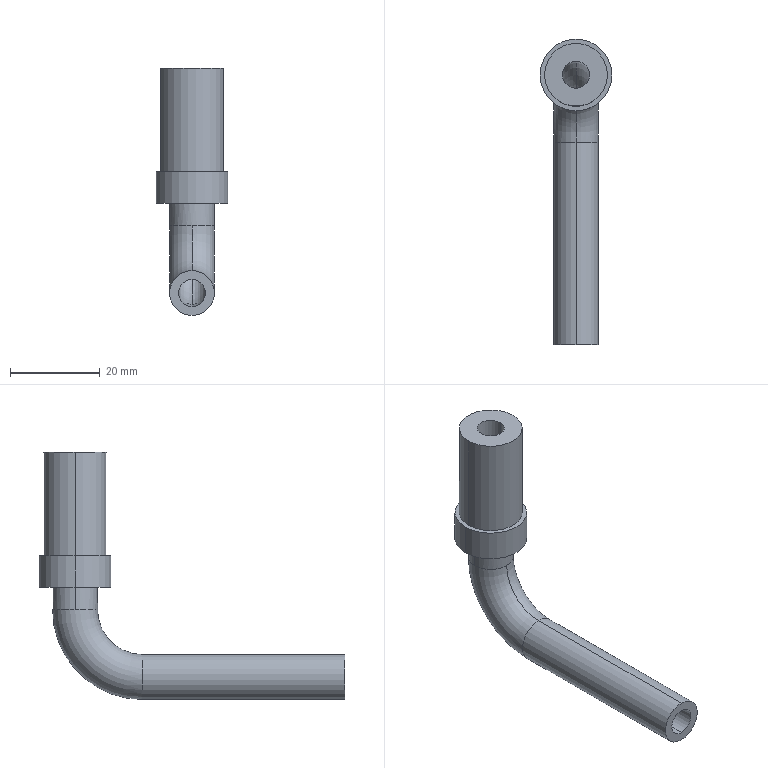Part | SolidWorks | features ICE 2, Sweep 1 | 1 solid | 20 faces | box 16 x 68 x 55 mm | volume 7797 mm3 | cylinder 12 | torus 4 | plane 4 | commonest cylinder face diameters 6 x4 10 x4 14 x2 16 x2
STEP:
#1=CARTESIAN_POINT('',(0.,3.,-35.));
#2=VERTEX_POINT('',#1);
#3=CARTESIAN_POINT('',(3.,0.,-35.));
#4=VERTEX_POINT('',#3);
#5=CARTESIAN_POINT('',(0.,0.,-35.));
#6=DIRECTION('',(0.,0.,-1.));
#7=DIRECTION('',(1.,0.,0.));
#8=AXIS2_PLACEMENT_3D('',#5,#6,#7);
#9=CIRCLE('',#8,3.);
#10=EDGE_CURVE('',#2,#4,#9,.T.);
#11=ORIENTED_EDGE('',*,*,#10,.F.);
#12=CARTESIAN_POINT('',(0.,-15.,-53.));
#13=VERTEX_POINT('',#12);
#14=CARTESIAN_POINT('',(0.,-15.,-35.));
#15=DIRECTION('',(-1.,0.,0.));
#16=DIRECTION('',(0.,0.,1.));
#17=AXIS2_PLACEMENT_3D('',#14,#15,#16);
#18=CIRCLE('',#17,18.);
#19=EDGE_CURVE('',#2,#13,#18,.T.);
#20=ORIENTED_EDGE('',*,*,#19,.T.);
#21=CARTESIAN_POINT('',(0.,-15.,-47.));
#22=VERTEX_POINT('',#21);
#23=CARTESIAN_POINT('',(0.,-15.,-50.));
#24=DIRECTION('',(0.,-1.,0.));
#25=DIRECTION('',(1.,0.,0.));
#26=AXIS2_PLACEMENT_3D('',#23,#24,#25);
#27=CIRCLE('',#26,3.);
#28=EDGE_CURVE('',#13,#22,#27,.T.);
#29=ORIENTED_EDGE('',*,*,#28,.T.);
#30=CARTESIAN_POINT('',(0.,-3.,-35.));
#31=VERTEX_POINT('',#30);
#32=CARTESIAN_POINT('',(0.,-15.,-35.));
#33=DIRECTION('',(-1.,0.,0.));
#34=DIRECTION('',(0.,0.,1.));
#35=AXIS2_PLACEMENT_3D('',#32,#33,#34);
#36=CIRCLE('',#35,12.);
#37=EDGE_CURVE('',#31,#22,#36,.T.);
#38=ORIENTED_EDGE('',*,*,#37,.F.);
#39=CARTESIAN_POINT('',(0.,0.,-35.));
#40=DIRECTION('',(0.,0.,-1.));
#41=DIRECTION('',(1.,0.,0.));
#42=AXIS2_PLACEMENT_3D('',#39,#40,#41);
#43=CIRCLE('',#42,3.);
#44=EDGE_CURVE('',#4,#31,#43,.T.);
#45=ORIENTED_EDGE('',*,*,#44,.F.);
#46=EDGE_LOOP('',(#11,#20,#29,#38,#45));
#47=FACE_OUTER_BOUND('',#46,.T.);
#48=CARTESIAN_POINT('',(0.,-15.,-35.));
#49=DIRECTION('',(-1.,0.,0.));
#50=DIRECTION('',(0.,0.,1.));
#51=AXIS2_PLACEMENT_3D('',#48,#49,#50);
#52=TOROIDAL_SURFACE('',#51,15.,3.);
#53=ADVANCED_FACE('',(#47),#52,.F.);
#54=CARTESIAN_POINT('',(0.,5.,-35.));
#55=VERTEX_POINT('',#54);
#56=CARTESIAN_POINT('',(-5.,0.,-35.));
#57=VERTEX_POINT('',#56);
#58=CARTESIAN_POINT('',(0.,0.,-35.));
#59=DIRECTION('',(0.,0.,1.));
#60=DIRECTION('',(1.,0.,0.));
#61=AXIS2_PLACEMENT_3D('',#58,#59,#60);
#62=CIRCLE('',#61,5.);
#63=EDGE_CURVE('',#55,#57,#62,.T.);
#64=ORIENTED_EDGE('',*,*,#63,.F.);
#65=CARTESIAN_POINT('',(0.,-15.,-55.));
#66=VERTEX_POINT('',#65);
#67=CARTESIAN_POINT('',(0.,-15.,-35.));
#68=DIRECTION('',(-1.,0.,0.));
#69=DIRECTION('',(0.,0.,1.));
#70=AXIS2_PLACEMENT_3D('',#67,#68,#69);
#71=CIRCLE('',#70,20.);
#72=EDGE_CURVE('',#55,#66,#71,.T.);
#73=ORIENTED_EDGE('',*,*,#72,.T.);
#74=CARTESIAN_POINT('',(0.,-15.,-45.));
#75=VERTEX_POINT('',#74);
#76=CARTESIAN_POINT('',(0.,-15.,-50.));
#77=DIRECTION('',(0.,1.,0.));
#78=DIRECTION('',(1.,0.,0.));
#79=AXIS2_PLACEMENT_3D('',#76,#77,#78);
#80=CIRCLE('',#79,5.);
#81=EDGE_CURVE('',#66,#75,#80,.T.);
#82=ORIENTED_EDGE('',*,*,#81,.T.);
#83=CARTESIAN_POINT('',(0.,-5.,-35.));
#84=VERTEX_POINT('',#83);
#85=CARTESIAN_POINT('',(0.,-15.,-35.));
#86=DIRECTION('',(-1.,0.,0.));
#87=DIRECTION('',(0.,0.,1.));
#88=AXIS2_PLACEMENT_3D('',#85,#86,#87);
#89=CIRCLE('',#88,10.);
#90=EDGE_CURVE('',#84,#75,#89,.T.);
#91=ORIENTED_EDGE('',*,*,#90,.F.);
#92=CARTESIAN_POINT('',(0.,0.,-35.));
#93=DIRECTION('',(0.,0.,1.));
#94=DIRECTION('',(1.,0.,0.));
#95=AXIS2_PLACEMENT_3D('',#92,#93,#94);
#96=CIRCLE('',#95,5.);
#97=EDGE_CURVE('',#57,#84,#96,.T.);
#98=ORIENTED_EDGE('',*,*,#97,.F.);
#99=EDGE_LOOP('',(#64,#73,#82,#91,#98));
#100=FACE_OUTER_BOUND('',#99,.T.);
#101=CARTESIAN_POINT('',(0.,-15.,-35.));
#102=DIRECTION('',(-1.,0.,0.));
#103=DIRECTION('',(0.,0.,1.));
#104=AXIS2_PLACEMENT_3D('',#101,#102,#103);
#105=TOROIDAL_SURFACE('',#104,15.,5.);
#106=ADVANCED_FACE('',(#100),#105,.T.);
#107=CARTESIAN_POINT('',(-8.,0.,-23.));
#108=VERTEX_POINT('',#107);
#109=CARTESIAN_POINT('',(8.,0.,-23.));
#110=VERTEX_POINT('',#109);
#111=CARTESIAN_POINT('',(0.,0.,-23.));
#112=DIRECTION('',(0.,0.,-1.));
#113=DIRECTION('',(-1.,0.,0.));
#114=AXIS2_PLACEMENT_3D('',#111,#112,#113);
#115=CIRCLE('',#114,8.);
#116=EDGE_CURVE('',#108,#110,#115,.T.);
#117=ORIENTED_EDGE('',*,*,#116,.T.);
#118=CARTESIAN_POINT('',(8.,0.,-30.));
#119=VERTEX_POINT('',#118);
#120=CARTESIAN_POINT('',(8.,0.,-23.));
#121=DIRECTION('',(0.,0.,-1.));
#122=VECTOR('',#121,1000.);
#123=LINE('',#120,#122);
#124=EDGE_CURVE('',#110,#119,#123,.T.);
#125=ORIENTED_EDGE('',*,*,#124,.T.);
#126=CARTESIAN_POINT('',(-8.,0.,-30.));
#127=VERTEX_POINT('',#126);
#128=CARTESIAN_POINT('',(0.,0.,-30.));
#129=DIRECTION('',(0.,0.,-1.));
#130=DIRECTION('',(-1.,0.,0.));
#131=AXIS2_PLACEMENT_3D('',#128,#129,#130);
#132=CIRCLE('',#131,8.);
#133=EDGE_CURVE('',#127,#119,#132,.T.);
#134=ORIENTED_EDGE('',*,*,#133,.F.);
#135=CARTESIAN_POINT('',(-8.,0.,-23.));
#136=DIRECTION('',(0.,0.,-1.));
#137=VECTOR('',#136,1000.);
#138=LINE('',#135,#137);
#139=EDGE_CURVE('',#108,#127,#138,.T.);
#140=ORIENTED_EDGE('',*,*,#139,.F.);
#141=EDGE_LOOP('',(#117,#125,#134,#140));
#142=FACE_OUTER_BOUND('',#141,.T.);
#143=CARTESIAN_POINT('',(0.,0.,-23.));
#144=DIRECTION('',(0.,0.,-1.));
#145=DIRECTION('',(-1.,0.,0.));
#146=AXIS2_PLACEMENT_3D('',#143,#144,#145);
#147=CYLINDRICAL_SURFACE('',#146,8.);
#148=ADVANCED_FACE('',(#142),#147,.T.);
#149=CARTESIAN_POINT('',(0.,-15.,-50.));
#150=DIRECTION('',(0.,-1.,0.));
#151=DIRECTION('',(1.,0.,0.));
#152=AXIS2_PLACEMENT_3D('',#149,#150,#151);
#153=CIRCLE('',#152,3.);
#154=EDGE_CURVE('',#22,#13,#153,.T.);
#155=ORIENTED_EDGE('',*,*,#154,.F.);
#156=CARTESIAN_POINT('',(0.,-60.,-47.));
#157=VERTEX_POINT('',#156);
#158=CARTESIAN_POINT('',(0.,-15.,-47.));
#159=DIRECTION('',(0.,-1.,0.));
#160=VECTOR('',#159,1000.);
#161=LINE('',#158,#160);
#162=EDGE_CURVE('',#22,#157,#161,.T.);
#163=ORIENTED_EDGE('',*,*,#162,.T.);
#164=CARTESIAN_POINT('',(0.,-60.,-53.));
#165=VERTEX_POINT('',#164);
#166=CARTESIAN_POINT('',(0.,-60.,-50.));
#167=DIRECTION('',(0.,-1.,0.));
#168=DIRECTION('',(1.,0.,0.));
#169=AXIS2_PLACEMENT_3D('',#166,#167,#168);
#170=CIRCLE('',#169,3.);
#171=EDGE_CURVE('',#157,#165,#170,.T.);
#172=ORIENTED_EDGE('',*,*,#171,.T.);
#173=CARTESIAN_POINT('',(0.,-15.,-53.));
#174=DIRECTION('',(0.,-1.,0.));
#175=VECTOR('',#174,1000.);
#176=LINE('',#173,#175);
#177=EDGE_CURVE('',#13,#165,#176,.T.);
#178=ORIENTED_EDGE('',*,*,#177,.F.);
#179=EDGE_LOOP('',(#155,#163,#172,#178));
#180=FACE_OUTER_BOUND('',#179,.T.);
#181=CARTESIAN_POINT('',(0.,-15.,-50.));
#182=DIRECTION('',(0.,-1.,0.));
#183=DIRECTION('',(0.,0.,-1.));
#184=AXIS2_PLACEMENT_3D('',#181,#182,#183);
#185=CYLINDRICAL_SURFACE('',#184,3.);
#186=ADVANCED_FACE('',(#180),#185,.F.);
#187=CARTESIAN_POINT('',(3.,0.,0.));
#188=VERTEX_POINT('',#187);
#189=CARTESIAN_POINT('',(-3.,0.,0.));
#190=VERTEX_POINT('',#189);
#191=CARTESIAN_POINT('',(0.,0.,0.));
#192=DIRECTION('',(0.,0.,-1.));
#193=DIRECTION('',(1.,0.,0.));
#194=AXIS2_PLACEMENT_3D('',#191,#192,#193);
#195=CIRCLE('',#194,3.);
#196=EDGE_CURVE('',#188,#190,#195,.T.);
#197=ORIENTED_EDGE('',*,*,#196,.F.);
#198=CARTESIAN_POINT('',(3.,0.,0.));
#199=DIRECTION('',(0.,0.,-1.));
#200=VECTOR('',#199,1000.);
#201=LINE('',#198,#200);
#202=EDGE_CURVE('',#188,#4,#201,.T.);
#203=ORIENTED_EDGE('',*,*,#202,.T.);
#204=ORIENTED_EDGE('',*,*,#44,.T.);
#205=CARTESIAN_POINT('',(-3.,0.,-35.));
#206=VERTEX_POINT('',#205);
#207=CARTESIAN_POINT('',(0.,0.,-35.));
#208=DIRECTION('',(0.,0.,-1.));
#209=DIRECTION('',(1.,0.,0.));
#210=AXIS2_PLACEMENT_3D('',#207,#208,#209);
#211=CIRCLE('',#210,3.);
#212=EDGE_CURVE('',#31,#206,#211,.T.);
#213=ORIENTED_EDGE('',*,*,#212,.T.);
#214=CARTESIAN_POINT('',(-3.,0.,0.));
#215=DIRECTION('',(0.,0.,-1.));
#216=VECTOR('',#215,1000.);
#217=LINE('',#214,#216);
#218=EDGE_CURVE('',#190,#206,#217,.T.);
#219=ORIENTED_EDGE('',*,*,#218,.F.);
#220=EDGE_LOOP('',(#197,#203,#204,#213,#219));
#221=FACE_OUTER_BOUND('',#220,.T.);
#222=CARTESIAN_POINT('',(0.,0.,0.));
#223=DIRECTION('',(0.,0.,-1.));
#224=DIRECTION('',(-1.,0.,0.));
#225=AXIS2_PLACEMENT_3D('',#222,#223,#224);
#226=CYLINDRICAL_SURFACE('',#225,3.);
#227=ADVANCED_FACE('',(#221),#226,.F.);
#228=CARTESIAN_POINT('',(0.,-15.,-50.));
#229=DIRECTION('',(0.,1.,0.));
#230=DIRECTION('',(1.,0.,0.));
#231=AXIS2_PLACEMENT_3D('',#228,#229,#230);
#232=CIRCLE('',#231,5.);
#233=EDGE_CURVE('',#75,#66,#232,.T.);
#234=ORIENTED_EDGE('',*,*,#233,.F.);
#235=CARTESIAN_POINT('',(0.,-60.,-45.));
#236=VERTEX_POINT('',#235);
#237=CARTESIAN_POINT('',(0.,-15.,-45.));
#238=DIRECTION('',(0.,-1.,0.));
#239=VECTOR('',#238,1000.);
#240=LINE('',#237,#239);
#241=EDGE_CURVE('',#75,#236,#240,.T.);
#242=ORIENTED_EDGE('',*,*,#241,.T.);
#243=CARTESIAN_POINT('',(0.,-60.,-55.));
#244=VERTEX_POINT('',#243);
#245=CARTESIAN_POINT('',(0.,-60.,-50.));
#246=DIRECTION('',(0.,1.,0.));
#247=DIRECTION('',(1.,0.,0.));
#248=AXIS2_PLACEMENT_3D('',#245,#246,#247);
#249=CIRCLE('',#248,5.);
#250=EDGE_CURVE('',#236,#244,#249,.T.);
#251=ORIENTED_EDGE('',*,*,#250,.T.);
#252=CARTESIAN_POINT('',(0.,-15.,-55.));
#253=DIRECTION('',(0.,-1.,0.));
#254=VECTOR('',#253,1000.);
#255=LINE('',#252,#254);
#256=EDGE_CURVE('',#66,#244,#255,.T.);
#257=ORIENTED_EDGE('',*,*,#256,.F.);
#258=EDGE_LOOP('',(#234,#242,#251,#257));
#259=FACE_OUTER_BOUND('',#258,.T.);
#260=CARTESIAN_POINT('',(0.,-15.,-50.));
#261=DIRECTION('',(0.,-1.,0.));
#262=DIRECTION('',(0.,0.,-1.));
#263=AXIS2_PLACEMENT_3D('',#260,#261,#262);
#264=CYLINDRICAL_SURFACE('',#263,5.);
#265=ADVANCED_FACE('',(#259),#264,.T.);
#266=CARTESIAN_POINT('',(5.,0.,-30.));
#267=VERTEX_POINT('',#266);
#268=CARTESIAN_POINT('',(-5.,0.,-30.));
#269=VERTEX_POINT('',#268);
#270=CARTESIAN_POINT('',(0.,0.,-30.));
#271=DIRECTION('',(0.,0.,1.));
#272=DIRECTION('',(1.,0.,0.));
#273=AXIS2_PLACEMENT_3D('',#270,#271,#272);
#274=CIRCLE('',#273,5.);
#275=EDGE_CURVE('',#267,#269,#274,.T.);
#276=ORIENTED_EDGE('',*,*,#275,.F.);
#277=CARTESIAN_POINT('',(5.,0.,-35.));
#278=VERTEX_POINT('',#277);
#279=CARTESIAN_POINT('',(5.,0.,0.));
#280=DIRECTION('',(0.,0.,-1.));
#281=VECTOR('',#280,1000.);
#282=LINE('',#279,#281);
#283=EDGE_CURVE('',#267,#278,#282,.T.);
#284=ORIENTED_EDGE('',*,*,#283,.T.);
#285=CARTESIAN_POINT('',(0.,0.,-35.));
#286=DIRECTION('',(0.,0.,1.));
#287=DIRECTION('',(1.,0.,0.));
#288=AXIS2_PLACEMENT_3D('',#285,#286,#287);
#289=CIRCLE('',#288,5.);
#290=EDGE_CURVE('',#278,#55,#289,.T.);
#291=ORIENTED_EDGE('',*,*,#290,.T.);
#292=ORIENTED_EDGE('',*,*,#63,.T.);
#293=CARTESIAN_POINT('',(-5.,0.,0.));
#294=DIRECTION('',(0.,0.,-1.));
#295=VECTOR('',#294,1000.);
#296=LINE('',#293,#295);
#297=EDGE_CURVE('',#269,#57,#296,.T.);
#298=ORIENTED_EDGE('',*,*,#297,.F.);
#299=EDGE_LOOP('',(#276,#284,#291,#292,#298));
#300=FACE_OUTER_BOUND('',#299,.T.);
#301=CARTESIAN_POINT('',(0.,0.,0.));
#302=DIRECTION('',(0.,0.,-1.));
#303=DIRECTION('',(-1.,0.,0.));
#304=AXIS2_PLACEMENT_3D('',#301,#302,#303);
#305=CYLINDRICAL_SURFACE('',#304,5.);
#306=ADVANCED_FACE('',(#300),#305,.T.);
#307=CARTESIAN_POINT('',(-7.,0.,-23.));
#308=VERTEX_POINT('',#307);
#309=CARTESIAN_POINT('',(7.,0.,-23.));
#310=VERTEX_POINT('',#309);
#311=CARTESIAN_POINT('',(0.,0.,-23.));
#312=DIRECTION('',(0.,0.,-1.));
#313=DIRECTION('',(-1.,0.,0.));
#314=AXIS2_PLACEMENT_3D('',#311,#312,#313);
#315=CIRCLE('',#314,7.);
#316=EDGE_CURVE('',#308,#310,#315,.T.);
#317=ORIENTED_EDGE('',*,*,#316,.F.);
#318=CARTESIAN_POINT('',(-7.,0.,0.));
#319=VERTEX_POINT('',#318);
#320=CARTESIAN_POINT('',(-7.,0.,-30.));
#321=DIRECTION('',(0.,0.,1.));
#322=VECTOR('',#321,1000.);
#323=LINE('',#320,#322);
#324=EDGE_CURVE('',#308,#319,#323,.T.);
#325=ORIENTED_EDGE('',*,*,#324,.T.);
#326=CARTESIAN_POINT('',(7.,0.,0.));
#327=VERTEX_POINT('',#326);
#328=CARTESIAN_POINT('',(0.,0.,0.));
#329=DIRECTION('',(0.,0.,1.));
#330=DIRECTION('',(1.,0.,0.));
#331=AXIS2_PLACEMENT_3D('',#328,#329,#330);
#332=CIRCLE('',#331,7.);
#333=EDGE_CURVE('',#327,#319,#332,.T.);
#334=ORIENTED_EDGE('',*,*,#333,.F.);
#335=CARTESIAN_POINT('',(7.,0.,-30.));
#336=DIRECTION('',(0.,0.,1.));
#337=VECTOR('',#336,1000.);
#338=LINE('',#335,#337);
#339=EDGE_CURVE('',#310,#327,#338,.T.);
#340=ORIENTED_EDGE('',*,*,#339,.F.);
#341=EDGE_LOOP('',(#317,#325,#334,#340));
#342=FACE_OUTER_BOUND('',#341,.T.);
#343=CARTESIAN_POINT('',(0.,0.,-30.));
#344=DIRECTION('',(0.,0.,1.));
#345=DIRECTION('',(1.,0.,0.));
#346=AXIS2_PLACEMENT_3D('',#343,#344,#345);
#347=CYLINDRICAL_SURFACE('',#346,7.);
#348=ADVANCED_FACE('',(#342),#347,.T.);
#349=ORIENTED_EDGE('',*,*,#324,.F.);
#350=CARTESIAN_POINT('',(0.,0.,-23.));
#351=DIRECTION('',(0.,0.,-1.));
#352=DIRECTION('',(-1.,0.,0.));
#353=AXIS2_PLACEMENT_3D('',#350,#351,#352);
#354=CIRCLE('',#353,7.);
#355=EDGE_CURVE('',#310,#308,#354,.T.);
#356=ORIENTED_EDGE('',*,*,#355,.F.);
#357=ORIENTED_EDGE('',*,*,#339,.T.);
#358=CARTESIAN_POINT('',(0.,0.,0.));
#359=DIRECTION('',(0.,0.,1.));
#360=DIRECTION('',(1.,0.,0.));
#361=AXIS2_PLACEMENT_3D('',#358,#359,#360);
#362=CIRCLE('',#361,7.);
#363=EDGE_CURVE('',#319,#327,#362,.T.);
#364=ORIENTED_EDGE('',*,*,#363,.F.);
#365=EDGE_LOOP('',(#349,#356,#357,#364));
#366=FACE_OUTER_BOUND('',#365,.T.);
#367=CARTESIAN_POINT('',(0.,0.,-30.));
#368=DIRECTION('',(0.,0.,1.));
#369=DIRECTION('',(1.,0.,0.));
#370=AXIS2_PLACEMENT_3D('',#367,#368,#369);
#371=CYLINDRICAL_SURFACE('',#370,7.);
#372=ADVANCED_FACE('',(#366),#371,.T.);
#373=ORIENTED_EDGE('',*,*,#283,.F.);
#374=CARTESIAN_POINT('',(0.,0.,-30.));
#375=DIRECTION('',(0.,0.,1.));
#376=DIRECTION('',(1.,0.,0.));
#377=AXIS2_PLACEMENT_3D('',#374,#375,#376);
#378=CIRCLE('',#377,5.);
#379=EDGE_CURVE('',#269,#267,#378,.T.);
#380=ORIENTED_EDGE('',*,*,#379,.F.);
#381=ORIENTED_EDGE('',*,*,#297,.T.);
#382=ORIENTED_EDGE('',*,*,#97,.T.);
#383=CARTESIAN_POINT('',(0.,0.,-35.));
#384=DIRECTION('',(0.,0.,1.));
#385=DIRECTION('',(1.,0.,0.));
#386=AXIS2_PLACEMENT_3D('',#383,#384,#385);
#387=CIRCLE('',#386,5.);
#388=EDGE_CURVE('',#84,#278,#387,.T.);
#389=ORIENTED_EDGE('',*,*,#388,.T.);
#390=EDGE_LOOP('',(#373,#380,#381,#382,#389));
#391=FACE_OUTER_BOUND('',#390,.T.);
#392=CARTESIAN_POINT('',(0.,0.,0.));
#393=DIRECTION('',(0.,0.,-1.));
#394=DIRECTION('',(-1.,0.,0.));
#395=AXIS2_PLACEMENT_3D('',#392,#393,#394);
#396=CYLINDRICAL_SURFACE('',#395,5.);
#397=ADVANCED_FACE('',(#391),#396,.T.);
#398=ORIENTED_EDGE('',*,*,#162,.F.);
#399=ORIENTED_EDGE('',*,*,#28,.F.);
#400=ORIENTED_EDGE('',*,*,#177,.T.);
#401=CARTESIAN_POINT('',(0.,-60.,-50.));
#402=DIRECTION('',(0.,-1.,0.));
#403=DIRECTION('',(1.,0.,0.));
#404=AXIS2_PLACEMENT_3D('',#401,#402,#403);
#405=CIRCLE('',#404,3.);
#406=EDGE_CURVE('',#165,#157,#405,.T.);
#407=ORIENTED_EDGE('',*,*,#406,.T.);
#408=EDGE_LOOP('',(#398,#399,#400,#407));
#409=FACE_OUTER_BOUND('',#408,.T.);
#410=CARTESIAN_POINT('',(0.,-15.,-50.));
#411=DIRECTION('',(0.,-1.,0.));
#412=DIRECTION('',(0.,0.,-1.));
#413=AXIS2_PLACEMENT_3D('',#410,#411,#412);
#414=CYLINDRICAL_SURFACE('',#413,3.);
#415=ADVANCED_FACE('',(#409),#414,.F.);
#416=ORIENTED_EDGE('',*,*,#19,.F.);
#417=CARTESIAN_POINT('',(0.,0.,-35.));
#418=DIRECTION('',(0.,0.,-1.));
#419=DIRECTION('',(1.,0.,0.));
#420=AXIS2_PLACEMENT_3D('',#417,#418,#419);
#421=CIRCLE('',#420,3.);
#422=EDGE_CURVE('',#206,#2,#421,.T.);
#423=ORIENTED_EDGE('',*,*,#422,.F.);
#424=ORIENTED_EDGE('',*,*,#212,.F.);
#425=ORIENTED_EDGE('',*,*,#37,.T.);
#426=ORIENTED_EDGE('',*,*,#154,.T.);
#427=EDGE_LOOP('',(#416,#423,#424,#425,#426));
#428=FACE_OUTER_BOUND('',#427,.T.);
#429=CARTESIAN_POINT('',(0.,-15.,-35.));
#430=DIRECTION('',(-1.,0.,0.));
#431=DIRECTION('',(0.,0.,1.));
#432=AXIS2_PLACEMENT_3D('',#429,#430,#431);
#433=TOROIDAL_SURFACE('',#432,15.,3.);
#434=ADVANCED_FACE('',(#428),#433,.F.);
#435=ORIENTED_EDGE('',*,*,#202,.F.);
#436=CARTESIAN_POINT('',(0.,0.,0.));
#437=DIRECTION('',(0.,0.,-1.));
#438=DIRECTION('',(1.,0.,0.));
#439=AXIS2_PLACEMENT_3D('',#436,#437,#438);
#440=CIRCLE('',#439,3.);
#441=EDGE_CURVE('',#190,#188,#440,.T.);
#442=ORIENTED_EDGE('',*,*,#441,.F.);
#443=ORIENTED_EDGE('',*,*,#218,.T.);
#444=ORIENTED_EDGE('',*,*,#422,.T.);
#445=ORIENTED_EDGE('',*,*,#10,.T.);
#446=EDGE_LOOP('',(#435,#442,#443,#444,#445));
#447=FACE_OUTER_BOUND('',#446,.T.);
#448=CARTESIAN_POINT('',(0.,0.,0.));
#449=DIRECTION('',(0.,0.,-1.));
#450=DIRECTION('',(-1.,0.,0.));
#451=AXIS2_PLACEMENT_3D('',#448,#449,#450);
#452=CYLINDRICAL_SURFACE('',#451,3.);
#453=ADVANCED_FACE('',(#447),#452,.F.);
#454=ORIENTED_EDGE('',*,*,#406,.F.);
#455=ORIENTED_EDGE('',*,*,#171,.F.);
#456=EDGE_LOOP('',(#454,#455));
#457=FACE_BOUND('',#456,.T.);
#458=CARTESIAN_POINT('',(0.,-60.,-50.));
#459=DIRECTION('',(0.,1.,0.));
#460=DIRECTION('',(1.,0.,0.));
#461=AXIS2_PLACEMENT_3D('',#458,#459,#460);
#462=CIRCLE('',#461,5.);
#463=EDGE_CURVE('',#244,#236,#462,.T.);
#464=ORIENTED_EDGE('',*,*,#463,.F.);
#465=ORIENTED_EDGE('',*,*,#250,.F.);
#466=EDGE_LOOP('',(#464,#465));
#467=FACE_OUTER_BOUND('',#466,.T.);
#468=CARTESIAN_POINT('',(0.,-60.,-50.));
#469=DIRECTION('',(0.,1.,0.));
#470=DIRECTION('',(1.,0.,0.));
#471=AXIS2_PLACEMENT_3D('',#468,#469,#470);
#472=PLANE('',#471);
#473=ADVANCED_FACE('',(#457,#467),#472,.F.);
#474=ORIENTED_EDGE('',*,*,#441,.T.);
#475=ORIENTED_EDGE('',*,*,#196,.T.);
#476=EDGE_LOOP('',(#474,#475));
#477=FACE_BOUND('',#476,.T.);
#478=ORIENTED_EDGE('',*,*,#333,.T.);
#479=ORIENTED_EDGE('',*,*,#363,.T.);
#480=EDGE_LOOP('',(#478,#479));
#481=FACE_OUTER_BOUND('',#480,.T.);
#482=CARTESIAN_POINT('',(0.,0.,0.));
#483=DIRECTION('',(0.,0.,1.));
#484=DIRECTION('',(1.,0.,0.));
#485=AXIS2_PLACEMENT_3D('',#482,#483,#484);
#486=PLANE('',#485);
#487=ADVANCED_FACE('',(#477,#481),#486,.T.);
#488=ORIENTED_EDGE('',*,*,#241,.F.);
#489=ORIENTED_EDGE('',*,*,#81,.F.);
#490=ORIENTED_EDGE('',*,*,#256,.T.);
#491=ORIENTED_EDGE('',*,*,#463,.T.);
#492=EDGE_LOOP('',(#488,#489,#490,#491));
#493=FACE_OUTER_BOUND('',#492,.T.);
#494=CARTESIAN_POINT('',(0.,-15.,-50.));
#495=DIRECTION('',(0.,-1.,0.));
#496=DIRECTION('',(0.,0.,-1.));
#497=AXIS2_PLACEMENT_3D('',#494,#495,#496);
#498=CYLINDRICAL_SURFACE('',#497,5.);
#499=ADVANCED_FACE('',(#493),#498,.T.);
#500=ORIENTED_EDGE('',*,*,#72,.F.);
#501=ORIENTED_EDGE('',*,*,#290,.F.);
#502=ORIENTED_EDGE('',*,*,#388,.F.);
#503=ORIENTED_EDGE('',*,*,#90,.T.);
#504=ORIENTED_EDGE('',*,*,#233,.T.);
#505=EDGE_LOOP('',(#500,#501,#502,#503,#504));
#506=FACE_OUTER_BOUND('',#505,.T.);
#507=CARTESIAN_POINT('',(0.,-15.,-35.));
#508=DIRECTION('',(-1.,0.,0.));
#509=DIRECTION('',(0.,0.,1.));
#510=AXIS2_PLACEMENT_3D('',#507,#508,#509);
#511=TOROIDAL_SURFACE('',#510,15.,5.);
#512=ADVANCED_FACE('',(#506),#511,.T.);
#513=ORIENTED_EDGE('',*,*,#379,.T.);
#514=ORIENTED_EDGE('',*,*,#275,.T.);
#515=EDGE_LOOP('',(#513,#514));
#516=FACE_BOUND('',#515,.T.);
#517=ORIENTED_EDGE('',*,*,#133,.T.);
#518=CARTESIAN_POINT('',(0.,0.,-30.));
#519=DIRECTION('',(0.,0.,-1.));
#520=DIRECTION('',(-1.,0.,0.));
#521=AXIS2_PLACEMENT_3D('',#518,#519,#520);
#522=CIRCLE('',#521,8.);
#523=EDGE_CURVE('',#119,#127,#522,.T.);
#524=ORIENTED_EDGE('',*,*,#523,.T.);
#525=EDGE_LOOP('',(#517,#524));
#526=FACE_OUTER_BOUND('',#525,.T.);
#527=CARTESIAN_POINT('',(0.,0.,-30.));
#528=DIRECTION('',(0.,0.,1.));
#529=DIRECTION('',(1.,0.,0.));
#530=AXIS2_PLACEMENT_3D('',#527,#528,#529);
#531=PLANE('',#530);
#532=ADVANCED_FACE('',(#516,#526),#531,.F.);
#533=ORIENTED_EDGE('',*,*,#124,.F.);
#534=CARTESIAN_POINT('',(0.,0.,-23.));
#535=DIRECTION('',(0.,0.,-1.));
#536=DIRECTION('',(-1.,0.,0.));
#537=AXIS2_PLACEMENT_3D('',#534,#535,#536);
#538=CIRCLE('',#537,8.);
#539=EDGE_CURVE('',#110,#108,#538,.T.);
#540=ORIENTED_EDGE('',*,*,#539,.T.);
#541=ORIENTED_EDGE('',*,*,#139,.T.);
#542=ORIENTED_EDGE('',*,*,#523,.F.);
#543=EDGE_LOOP('',(#533,#540,#541,#542));
#544=FACE_OUTER_BOUND('',#543,.T.);
#545=CARTESIAN_POINT('',(0.,0.,-23.));
#546=DIRECTION('',(0.,0.,-1.));
#547=DIRECTION('',(-1.,0.,0.));
#548=AXIS2_PLACEMENT_3D('',#545,#546,#547);
#549=CYLINDRICAL_SURFACE('',#548,8.);
#550=ADVANCED_FACE('',(#544),#549,.T.);
#551=ORIENTED_EDGE('',*,*,#355,.T.);
#552=ORIENTED_EDGE('',*,*,#316,.T.);
#553=EDGE_LOOP('',(#551,#552));
#554=FACE_BOUND('',#553,.T.);
#555=ORIENTED_EDGE('',*,*,#116,.F.);
#556=ORIENTED_EDGE('',*,*,#539,.F.);
#557=EDGE_LOOP('',(#555,#556));
#558=FACE_OUTER_BOUND('',#557,.T.);
#559=CARTESIAN_POINT('',(0.,0.,-23.));
#560=DIRECTION('',(0.,0.,-1.));
#561=DIRECTION('',(-1.,0.,0.));
#562=AXIS2_PLACEMENT_3D('',#559,#560,#561);
#563=PLANE('',#562);
#564=ADVANCED_FACE('',(#554,#558),#563,.F.);
#565=CLOSED_SHELL('',(#53,#106,#148,#186,#227,#265,#306,#348,#372,#397,#415,#434,#453,#473,#487,#499,#512,#532,#550,#564));
#566=MANIFOLD_SOLID_BREP('',#565);
#567=CARTESIAN_POINT('',(0.,0.,0.));
#568=DIRECTION('',(0.,0.,1.));
#569=DIRECTION('',(1.,0.,0.));
#570=AXIS2_PLACEMENT_3D('',#567,#568,#569);
#571=(LENGTH_UNIT()NAMED_UNIT(*)SI_UNIT(.MILLI.,.METRE.));
#572=UNCERTAINTY_MEASURE_WITH_UNIT(LENGTH_MEASURE(0.00001),#571,'','');
#573=(NAMED_UNIT(*)PLANE_ANGLE_UNIT()SI_UNIT($,.RADIAN.));
#574=(NAMED_UNIT(*)SI_UNIT($,.STERADIAN.)SOLID_ANGLE_UNIT());
#575=(GEOMETRIC_REPRESENTATION_CONTEXT(3)GLOBAL_UNCERTAINTY_ASSIGNED_CONTEXT((#572))GLOBAL_UNIT_ASSIGNED_CONTEXT((#571,#573,#574))REPRESENTATION_CONTEXT('',''));
#576=ADVANCED_BREP_SHAPE_REPRESENTATION('',(#566,#570),#575);